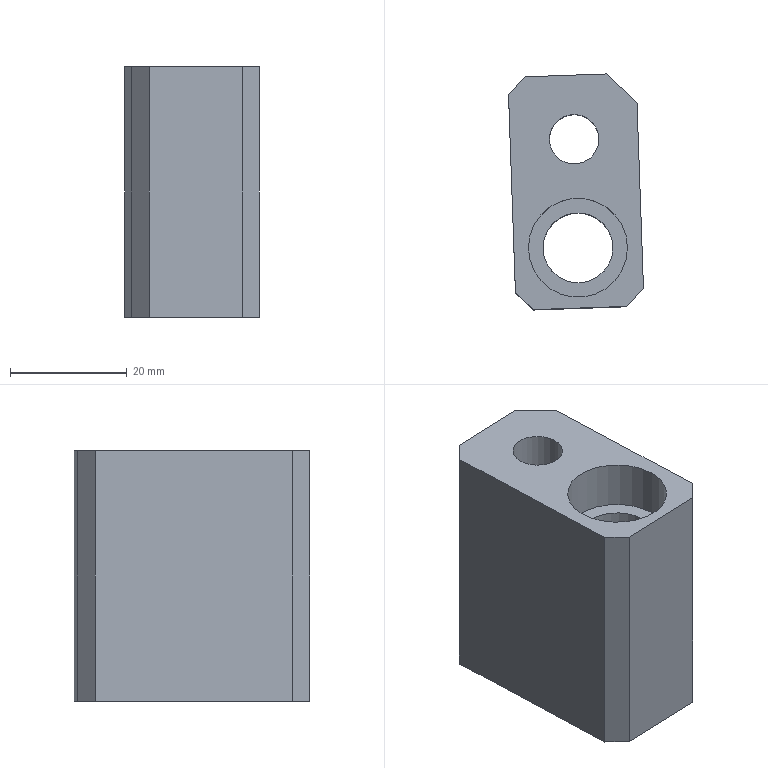Part | NX | features PH-8 2 | 1 solid | 16 faces | box 23.173 x 40.464 x 43 mm | volume 27281 mm3 | plane 12 | cylinder 4 | commonest cylinder face diameters 8.5 x1 12.001 x1 14.5 x1 17 x1
STEP:
#1=CARTESIAN_POINT('',(3121.766,-809.537,945.716));
#2=VERTEX_POINT('',#1);
#3=CARTESIAN_POINT('',(3113.266,-809.537,945.716));
#4=DIRECTION('',(0.,0.,1.));
#5=DIRECTION('',(1.,0.,0.));
#6=AXIS2_PLACEMENT_3D('',#3,#4,#5);
#7=CIRCLE('',#6,8.5);
#8=EDGE_CURVE('',#2,#2,#7,.F.);
#9=ORIENTED_EDGE('',*,*,#8,.T.);
#10=EDGE_LOOP('',(#9));
#11=FACE_BOUND('',#10,.T.);
#12=CARTESIAN_POINT('',(3116.862,-790.75,945.716));
#13=VERTEX_POINT('',#12);
#14=CARTESIAN_POINT('',(3112.615,-790.899,945.716));
#15=DIRECTION('',(0.,0.,1.));
#16=DIRECTION('',(0.9994,0.0349,0.));
#17=AXIS2_PLACEMENT_3D('',#14,#15,#16);
#18=CIRCLE('',#17,4.25);
#19=EDGE_CURVE('',#13,#13,#18,.T.);
#20=ORIENTED_EDGE('',*,*,#19,.F.);
#21=EDGE_LOOP('',(#20));
#22=FACE_BOUND('',#21,.T.);
#23=CARTESIAN_POINT('',(3123.399,-784.519,945.716));
#24=VERTEX_POINT('',#23);
#25=CARTESIAN_POINT('',(3124.515,-816.499,945.716));
#26=VERTEX_POINT('',#25);
#27=CARTESIAN_POINT('',(3123.922,-799.509,945.716));
#28=DIRECTION('',(0.0349,-0.9994,0.));
#29=VECTOR('',#28,1000.);
#30=LINE('',#27,#29);
#31=EDGE_CURVE('',#24,#26,#30,.T.);
#32=ORIENTED_EDGE('',*,*,#31,.F.);
#33=CARTESIAN_POINT('',(3118.227,-779.696,945.716));
#34=VERTEX_POINT('',#33);
#35=CARTESIAN_POINT('',(3124.433,-785.483,945.716));
#36=DIRECTION('',(0.7314,-0.682,0.));
#37=VECTOR('',#36,1000.);
#38=LINE('',#35,#37);
#39=EDGE_CURVE('',#24,#34,#38,.F.);
#40=ORIENTED_EDGE('',*,*,#39,.T.);
#41=CARTESIAN_POINT('',(3104.236,-780.185,945.716));
#42=VERTEX_POINT('',#41);
#43=CARTESIAN_POINT('',(3112.231,-779.905,945.716));
#44=DIRECTION('',(0.9994,0.0349,0.));
#45=VECTOR('',#44,1000.);
#46=LINE('',#43,#45);
#47=EDGE_CURVE('',#42,#34,#46,.T.);
#48=ORIENTED_EDGE('',*,*,#47,.F.);
#49=CARTESIAN_POINT('',(3101.342,-783.288,945.716));
#50=VERTEX_POINT('',#49);
#51=CARTESIAN_POINT('',(3099.413,-785.356,945.716));
#52=DIRECTION('',(0.682,0.7314,0.));
#53=VECTOR('',#52,1000.);
#54=LINE('',#51,#53);
#55=EDGE_CURVE('',#42,#50,#54,.F.);
#56=ORIENTED_EDGE('',*,*,#55,.T.);
#57=CARTESIAN_POINT('',(3102.529,-817.267,945.716));
#58=VERTEX_POINT('',#57);
#59=CARTESIAN_POINT('',(3101.936,-800.277,945.716));
#60=DIRECTION('',(-0.0349,0.9994,0.));
#61=VECTOR('',#60,1000.);
#62=LINE('',#59,#61);
#63=EDGE_CURVE('',#58,#50,#62,.T.);
#64=ORIENTED_EDGE('',*,*,#63,.F.);
#65=CARTESIAN_POINT('',(3105.632,-820.16,945.716));
#66=VERTEX_POINT('',#65);
#67=CARTESIAN_POINT('',(3099.426,-814.373,945.716));
#68=DIRECTION('',(-0.7314,0.682,0.));
#69=VECTOR('',#68,1000.);
#70=LINE('',#67,#69);
#71=EDGE_CURVE('',#58,#66,#70,.F.);
#72=ORIENTED_EDGE('',*,*,#71,.T.);
#73=CARTESIAN_POINT('',(3121.622,-819.602,945.716));
#74=VERTEX_POINT('',#73);
#75=CARTESIAN_POINT('',(3113.627,-819.881,945.716));
#76=DIRECTION('',(-0.9994,-0.0349,0.));
#77=VECTOR('',#76,1000.);
#78=LINE('',#75,#77);
#79=EDGE_CURVE('',#74,#66,#78,.T.);
#80=ORIENTED_EDGE('',*,*,#79,.F.);
#81=CARTESIAN_POINT('',(3127.409,-813.396,945.716));
#82=DIRECTION('',(-0.682,-0.7314,0.));
#83=VECTOR('',#82,1000.);
#84=LINE('',#81,#83);
#85=EDGE_CURVE('',#74,#26,#84,.F.);
#86=ORIENTED_EDGE('',*,*,#85,.T.);
#87=EDGE_LOOP('',(#32,#40,#48,#56,#64,#72,#80,#86));
#88=FACE_BOUND('',#87,.T.);
#89=CARTESIAN_POINT('',(3112.929,-799.893,945.716));
#90=DIRECTION('',(0.,0.,1.));
#91=DIRECTION('',(0.9994,0.0349,0.));
#92=AXIS2_PLACEMENT_3D('',#89,#90,#91);
#93=PLANE('',#92);
#94=ADVANCED_FACE('',(#11,#22,#88),#93,.T.);
#95=CARTESIAN_POINT('',(3105.632,-820.16,902.716));
#96=VERTEX_POINT('',#95);
#97=CARTESIAN_POINT('',(3121.622,-819.602,902.716));
#98=VERTEX_POINT('',#97);
#99=CARTESIAN_POINT('',(3113.627,-819.881,902.716));
#100=DIRECTION('',(0.9994,0.0349,0.));
#101=VECTOR('',#100,1000.);
#102=LINE('',#99,#101);
#103=EDGE_CURVE('',#96,#98,#102,.T.);
#104=ORIENTED_EDGE('',*,*,#103,.T.);
#105=CARTESIAN_POINT('',(3121.622,-819.602,920.716));
#106=DIRECTION('',(0.,0.,-1.));
#107=VECTOR('',#106,1000.);
#108=LINE('',#105,#107);
#109=EDGE_CURVE('',#98,#74,#108,.F.);
#110=ORIENTED_EDGE('',*,*,#109,.T.);
#111=ORIENTED_EDGE('',*,*,#79,.T.);
#112=CARTESIAN_POINT('',(3105.632,-820.16,920.716));
#113=DIRECTION('',(0.,0.,1.));
#114=VECTOR('',#113,1000.);
#115=LINE('',#112,#114);
#116=EDGE_CURVE('',#66,#96,#115,.F.);
#117=ORIENTED_EDGE('',*,*,#116,.T.);
#118=EDGE_LOOP('',(#104,#110,#111,#117));
#119=FACE_BOUND('',#118,.T.);
#120=CARTESIAN_POINT('',(3113.627,-819.881,920.716));
#121=DIRECTION('',(0.0349,-0.9994,0.));
#122=DIRECTION('',(0.,0.,-1.));
#123=AXIS2_PLACEMENT_3D('',#120,#121,#122);
#124=PLANE('',#123);
#125=ADVANCED_FACE('',(#119),#124,.T.);
#126=ORIENTED_EDGE('',*,*,#63,.T.);
#127=CARTESIAN_POINT('',(3101.342,-783.288,902.716));
#128=VERTEX_POINT('',#127);
#129=CARTESIAN_POINT('',(3101.342,-783.288,920.716));
#130=DIRECTION('',(0.,0.,-1.));
#131=VECTOR('',#130,1000.);
#132=LINE('',#129,#131);
#133=EDGE_CURVE('',#50,#128,#132,.T.);
#134=ORIENTED_EDGE('',*,*,#133,.T.);
#135=CARTESIAN_POINT('',(3102.529,-817.267,902.716));
#136=VERTEX_POINT('',#135);
#137=CARTESIAN_POINT('',(3101.936,-800.277,902.716));
#138=DIRECTION('',(0.0349,-0.9994,0.));
#139=VECTOR('',#138,1000.);
#140=LINE('',#137,#139);
#141=EDGE_CURVE('',#128,#136,#140,.T.);
#142=ORIENTED_EDGE('',*,*,#141,.T.);
#143=CARTESIAN_POINT('',(3102.529,-817.267,920.716));
#144=DIRECTION('',(0.,0.,-1.));
#145=VECTOR('',#144,1000.);
#146=LINE('',#143,#145);
#147=EDGE_CURVE('',#136,#58,#146,.F.);
#148=ORIENTED_EDGE('',*,*,#147,.T.);
#149=EDGE_LOOP('',(#126,#134,#142,#148));
#150=FACE_BOUND('',#149,.T.);
#151=CARTESIAN_POINT('',(3101.936,-800.277,920.716));
#152=DIRECTION('',(-0.9994,-0.0349,0.));
#153=DIRECTION('',(0.,0.,1.));
#154=AXIS2_PLACEMENT_3D('',#151,#152,#153);
#155=PLANE('',#154);
#156=ADVANCED_FACE('',(#150),#155,.T.);
#157=ORIENTED_EDGE('',*,*,#47,.T.);
#158=CARTESIAN_POINT('',(3118.227,-779.696,902.716));
#159=VERTEX_POINT('',#158);
#160=CARTESIAN_POINT('',(3118.227,-779.696,920.716));
#161=DIRECTION('',(0.,0.,-1.));
#162=VECTOR('',#161,1000.);
#163=LINE('',#160,#162);
#164=EDGE_CURVE('',#34,#159,#163,.T.);
#165=ORIENTED_EDGE('',*,*,#164,.T.);
#166=CARTESIAN_POINT('',(3104.236,-780.185,902.716));
#167=VERTEX_POINT('',#166);
#168=CARTESIAN_POINT('',(3112.231,-779.905,902.716));
#169=DIRECTION('',(-0.9994,-0.0349,0.));
#170=VECTOR('',#169,1000.);
#171=LINE('',#168,#170);
#172=EDGE_CURVE('',#159,#167,#171,.T.);
#173=ORIENTED_EDGE('',*,*,#172,.T.);
#174=CARTESIAN_POINT('',(3104.236,-780.185,920.716));
#175=DIRECTION('',(0.,0.,1.));
#176=VECTOR('',#175,1000.);
#177=LINE('',#174,#176);
#178=EDGE_CURVE('',#167,#42,#177,.T.);
#179=ORIENTED_EDGE('',*,*,#178,.T.);
#180=EDGE_LOOP('',(#157,#165,#173,#179));
#181=FACE_BOUND('',#180,.T.);
#182=CARTESIAN_POINT('',(3112.231,-779.905,920.716));
#183=DIRECTION('',(-0.0349,0.9994,0.));
#184=DIRECTION('',(0.,0.,1.));
#185=AXIS2_PLACEMENT_3D('',#182,#183,#184);
#186=PLANE('',#185);
#187=ADVANCED_FACE('',(#181),#186,.T.);
#188=CARTESIAN_POINT('',(3107.265,-809.537,902.716));
#189=VERTEX_POINT('',#188);
#190=CARTESIAN_POINT('',(3113.266,-809.537,902.716));
#191=DIRECTION('',(0.,0.,-1.));
#192=DIRECTION('',(-1.,0.,0.));
#193=AXIS2_PLACEMENT_3D('',#190,#191,#192);
#194=CIRCLE('',#193,6.);
#195=EDGE_CURVE('',#189,#189,#194,.T.);
#196=ORIENTED_EDGE('',*,*,#195,.F.);
#197=EDGE_LOOP('',(#196));
#198=FACE_BOUND('',#197,.T.);
#199=CARTESIAN_POINT('',(3105.365,-790.899,902.716));
#200=VERTEX_POINT('',#199);
#201=CARTESIAN_POINT('',(3112.615,-790.899,902.716));
#202=DIRECTION('',(0.,0.,-1.));
#203=DIRECTION('',(-1.,0.,0.));
#204=AXIS2_PLACEMENT_3D('',#201,#202,#203);
#205=CIRCLE('',#204,7.25);
#206=EDGE_CURVE('',#200,#200,#205,.F.);
#207=ORIENTED_EDGE('',*,*,#206,.T.);
#208=EDGE_LOOP('',(#207));
#209=FACE_BOUND('',#208,.T.);
#210=ORIENTED_EDGE('',*,*,#172,.F.);
#211=CARTESIAN_POINT('',(3123.399,-784.519,902.716));
#212=VERTEX_POINT('',#211);
#213=CARTESIAN_POINT('',(3125.467,-786.448,902.716));
#214=DIRECTION('',(-0.7314,0.682,0.));
#215=VECTOR('',#214,1000.);
#216=LINE('',#213,#215);
#217=EDGE_CURVE('',#159,#212,#216,.F.);
#218=ORIENTED_EDGE('',*,*,#217,.T.);
#219=CARTESIAN_POINT('',(3124.515,-816.499,902.716));
#220=VERTEX_POINT('',#219);
#221=CARTESIAN_POINT('',(3123.922,-799.509,902.716));
#222=DIRECTION('',(-0.0349,0.9994,0.));
#223=VECTOR('',#222,1000.);
#224=LINE('',#221,#223);
#225=EDGE_CURVE('',#220,#212,#224,.T.);
#226=ORIENTED_EDGE('',*,*,#225,.F.);
#227=CARTESIAN_POINT('',(3127.409,-813.396,902.716));
#228=DIRECTION('',(0.682,0.7314,0.));
#229=VECTOR('',#228,1000.);
#230=LINE('',#227,#229);
#231=EDGE_CURVE('',#220,#98,#230,.F.);
#232=ORIENTED_EDGE('',*,*,#231,.T.);
#233=ORIENTED_EDGE('',*,*,#103,.F.);
#234=CARTESIAN_POINT('',(3099.426,-814.373,902.716));
#235=DIRECTION('',(0.7314,-0.682,0.));
#236=VECTOR('',#235,1000.);
#237=LINE('',#234,#236);
#238=EDGE_CURVE('',#96,#136,#237,.F.);
#239=ORIENTED_EDGE('',*,*,#238,.T.);
#240=ORIENTED_EDGE('',*,*,#141,.F.);
#241=CARTESIAN_POINT('',(3098.449,-786.39,902.716));
#242=DIRECTION('',(-0.682,-0.7314,0.));
#243=VECTOR('',#242,1000.);
#244=LINE('',#241,#243);
#245=EDGE_CURVE('',#128,#167,#244,.F.);
#246=ORIENTED_EDGE('',*,*,#245,.T.);
#247=EDGE_LOOP('',(#210,#218,#226,#232,#233,#239,#240,#246));
#248=FACE_BOUND('',#247,.T.);
#249=CARTESIAN_POINT('',(3112.929,-799.893,902.716));
#250=DIRECTION('',(0.,0.,-1.));
#251=DIRECTION('',(-0.9994,-0.0349,0.));
#252=AXIS2_PLACEMENT_3D('',#249,#250,#251);
#253=PLANE('',#252);
#254=ADVANCED_FACE('',(#198,#209,#248),#253,.T.);
#255=ORIENTED_EDGE('',*,*,#225,.T.);
#256=CARTESIAN_POINT('',(3123.399,-784.519,920.716));
#257=DIRECTION('',(0.,0.,1.));
#258=VECTOR('',#257,1000.);
#259=LINE('',#256,#258);
#260=EDGE_CURVE('',#212,#24,#259,.T.);
#261=ORIENTED_EDGE('',*,*,#260,.T.);
#262=ORIENTED_EDGE('',*,*,#31,.T.);
#263=CARTESIAN_POINT('',(3124.515,-816.499,920.716));
#264=DIRECTION('',(0.,0.,1.));
#265=VECTOR('',#264,1000.);
#266=LINE('',#263,#265);
#267=EDGE_CURVE('',#26,#220,#266,.F.);
#268=ORIENTED_EDGE('',*,*,#267,.T.);
#269=EDGE_LOOP('',(#255,#261,#262,#268));
#270=FACE_BOUND('',#269,.T.);
#271=CARTESIAN_POINT('',(3123.922,-799.509,920.716));
#272=DIRECTION('',(0.9994,0.0349,0.));
#273=DIRECTION('',(0.,0.,-1.));
#274=AXIS2_PLACEMENT_3D('',#271,#272,#273);
#275=PLANE('',#274);
#276=ADVANCED_FACE('',(#270),#275,.T.);
#277=ORIENTED_EDGE('',*,*,#231,.F.);
#278=ORIENTED_EDGE('',*,*,#267,.F.);
#279=ORIENTED_EDGE('',*,*,#85,.F.);
#280=ORIENTED_EDGE('',*,*,#109,.F.);
#281=EDGE_LOOP('',(#277,#278,#279,#280));
#282=FACE_BOUND('',#281,.T.);
#283=CARTESIAN_POINT('',(3121.622,-819.602,920.716));
#284=DIRECTION('',(-0.7314,0.682,0.));
#285=DIRECTION('',(-0.682,-0.7314,0.));
#286=AXIS2_PLACEMENT_3D('',#283,#284,#285);
#287=PLANE('',#286);
#288=ADVANCED_FACE('',(#282),#287,.F.);
#289=ORIENTED_EDGE('',*,*,#238,.F.);
#290=ORIENTED_EDGE('',*,*,#116,.F.);
#291=ORIENTED_EDGE('',*,*,#71,.F.);
#292=ORIENTED_EDGE('',*,*,#147,.F.);
#293=EDGE_LOOP('',(#289,#290,#291,#292));
#294=FACE_BOUND('',#293,.T.);
#295=CARTESIAN_POINT('',(3102.529,-817.267,920.716));
#296=DIRECTION('',(0.682,0.7314,0.));
#297=DIRECTION('',(-0.7314,0.682,0.));
#298=AXIS2_PLACEMENT_3D('',#295,#296,#297);
#299=PLANE('',#298);
#300=ADVANCED_FACE('',(#294),#299,.F.);
#301=ORIENTED_EDGE('',*,*,#245,.F.);
#302=ORIENTED_EDGE('',*,*,#133,.F.);
#303=ORIENTED_EDGE('',*,*,#55,.F.);
#304=ORIENTED_EDGE('',*,*,#178,.F.);
#305=EDGE_LOOP('',(#301,#302,#303,#304));
#306=FACE_BOUND('',#305,.T.);
#307=CARTESIAN_POINT('',(3104.236,-780.185,920.716));
#308=DIRECTION('',(0.7314,-0.682,0.));
#309=DIRECTION('',(0.682,0.7314,0.));
#310=AXIS2_PLACEMENT_3D('',#307,#308,#309);
#311=PLANE('',#310);
#312=ADVANCED_FACE('',(#306),#311,.F.);
#313=CARTESIAN_POINT('',(3116.865,-790.899,913.716));
#314=VERTEX_POINT('',#313);
#315=CARTESIAN_POINT('',(3112.615,-790.899,913.716));
#316=DIRECTION('',(0.,0.,1.));
#317=DIRECTION('',(1.,0.,0.));
#318=AXIS2_PLACEMENT_3D('',#315,#316,#317);
#319=CIRCLE('',#318,4.25);
#320=EDGE_CURVE('',#314,#314,#319,.T.);
#321=ORIENTED_EDGE('',*,*,#320,.T.);
#322=EDGE_LOOP('',(#321));
#323=FACE_BOUND('',#322,.T.);
#324=CARTESIAN_POINT('',(3119.865,-790.899,913.716));
#325=VERTEX_POINT('',#324);
#326=CARTESIAN_POINT('',(3112.615,-790.899,913.716));
#327=DIRECTION('',(0.,0.,1.));
#328=DIRECTION('',(1.,0.,0.));
#329=AXIS2_PLACEMENT_3D('',#326,#327,#328);
#330=CIRCLE('',#329,7.25);
#331=EDGE_CURVE('',#325,#325,#330,.T.);
#332=ORIENTED_EDGE('',*,*,#331,.F.);
#333=EDGE_LOOP('',(#332));
#334=FACE_BOUND('',#333,.T.);
#335=CARTESIAN_POINT('',(3112.615,-790.899,913.716));
#336=DIRECTION('',(0.,0.,1.));
#337=DIRECTION('',(0.9994,0.0349,0.));
#338=AXIS2_PLACEMENT_3D('',#335,#336,#337);
#339=PLANE('',#338);
#340=ADVANCED_FACE('',(#323,#334),#339,.F.);
#341=ORIENTED_EDGE('',*,*,#206,.F.);
#342=EDGE_LOOP('',(#341));
#343=FACE_BOUND('',#342,.T.);
#344=ORIENTED_EDGE('',*,*,#331,.T.);
#345=EDGE_LOOP('',(#344));
#346=FACE_BOUND('',#345,.T.);
#347=CARTESIAN_POINT('',(3112.615,-790.899,931.716));
#348=DIRECTION('',(0.,0.,-1.));
#349=DIRECTION('',(0.9994,0.0349,0.));
#350=AXIS2_PLACEMENT_3D('',#347,#348,#349);
#351=CYLINDRICAL_SURFACE('',#350,7.25);
#352=ADVANCED_FACE('',(#343,#346),#351,.F.);
#353=ORIENTED_EDGE('',*,*,#19,.T.);
#354=EDGE_LOOP('',(#353));
#355=FACE_BOUND('',#354,.T.);
#356=ORIENTED_EDGE('',*,*,#320,.F.);
#357=EDGE_LOOP('',(#356));
#358=FACE_BOUND('',#357,.T.);
#359=CARTESIAN_POINT('',(3112.615,-790.899,946.716));
#360=DIRECTION('',(0.,0.,-1.));
#361=DIRECTION('',(0.9994,0.0349,0.));
#362=AXIS2_PLACEMENT_3D('',#359,#360,#361);
#363=CYLINDRICAL_SURFACE('',#362,4.25);
#364=ADVANCED_FACE('',(#355,#358),#363,.F.);
#365=ORIENTED_EDGE('',*,*,#195,.T.);
#366=EDGE_LOOP('',(#365));
#367=FACE_BOUND('',#366,.T.);
#368=CARTESIAN_POINT('',(3107.265,-809.537,937.416));
#369=VERTEX_POINT('',#368);
#370=CARTESIAN_POINT('',(3113.266,-809.537,937.416));
#371=DIRECTION('',(0.,0.,-1.));
#372=DIRECTION('',(-1.,0.,0.));
#373=AXIS2_PLACEMENT_3D('',#370,#371,#372);
#374=CIRCLE('',#373,6.);
#375=EDGE_CURVE('',#369,#369,#374,.T.);
#376=ORIENTED_EDGE('',*,*,#375,.F.);
#377=EDGE_LOOP('',(#376));
#378=FACE_BOUND('',#377,.T.);
#379=CARTESIAN_POINT('',(3113.266,-809.537,945.716));
#380=DIRECTION('',(0.,0.,-1.));
#381=DIRECTION('',(1.,0.,0.));
#382=AXIS2_PLACEMENT_3D('',#379,#380,#381);
#383=CYLINDRICAL_SURFACE('',#382,6.);
#384=ADVANCED_FACE('',(#367,#378),#383,.F.);
#385=ORIENTED_EDGE('',*,*,#375,.T.);
#386=EDGE_LOOP('',(#385));
#387=FACE_BOUND('',#386,.T.);
#388=CARTESIAN_POINT('',(3104.766,-809.537,937.416));
#389=VERTEX_POINT('',#388);
#390=CARTESIAN_POINT('',(3113.266,-809.537,937.416));
#391=DIRECTION('',(0.,0.,-1.));
#392=DIRECTION('',(-1.,0.,0.));
#393=AXIS2_PLACEMENT_3D('',#390,#391,#392);
#394=CIRCLE('',#393,8.5);
#395=EDGE_CURVE('',#389,#389,#394,.T.);
#396=ORIENTED_EDGE('',*,*,#395,.F.);
#397=EDGE_LOOP('',(#396));
#398=FACE_BOUND('',#397,.T.);
#399=CARTESIAN_POINT('',(3113.266,-809.537,937.416));
#400=DIRECTION('',(0.,0.,-1.));
#401=DIRECTION('',(-1.,0.,0.));
#402=AXIS2_PLACEMENT_3D('',#399,#400,#401);
#403=PLANE('',#402);
#404=ADVANCED_FACE('',(#387,#398),#403,.F.);
#405=ORIENTED_EDGE('',*,*,#395,.T.);
#406=EDGE_LOOP('',(#405));
#407=FACE_BOUND('',#406,.T.);
#408=ORIENTED_EDGE('',*,*,#8,.F.);
#409=EDGE_LOOP('',(#408));
#410=FACE_BOUND('',#409,.T.);
#411=CARTESIAN_POINT('',(3113.266,-809.537,945.716));
#412=DIRECTION('',(0.,0.,-1.));
#413=DIRECTION('',(1.,0.,0.));
#414=AXIS2_PLACEMENT_3D('',#411,#412,#413);
#415=CYLINDRICAL_SURFACE('',#414,8.5);
#416=ADVANCED_FACE('',(#407,#410),#415,.F.);
#417=ORIENTED_EDGE('',*,*,#39,.F.);
#418=ORIENTED_EDGE('',*,*,#260,.F.);
#419=ORIENTED_EDGE('',*,*,#217,.F.);
#420=ORIENTED_EDGE('',*,*,#164,.F.);
#421=EDGE_LOOP('',(#417,#418,#419,#420));
#422=FACE_BOUND('',#421,.T.);
#423=CARTESIAN_POINT('',(3118.227,-779.696,920.716));
#424=DIRECTION('',(-0.682,-0.7314,0.));
#425=DIRECTION('',(0.,0.,-1.));
#426=AXIS2_PLACEMENT_3D('',#423,#424,#425);
#427=PLANE('',#426);
#428=ADVANCED_FACE('',(#422),#427,.F.);
#429=CLOSED_SHELL('',(#94,#125,#156,#187,#254,#276,#288,#300,#312,#340,#352,#364,#384,#404,#416,#428));
#430=MANIFOLD_SOLID_BREP('',#429);
#431=(LENGTH_UNIT()NAMED_UNIT(*)SI_UNIT(.MILLI.,.METRE.));
#432=UNCERTAINTY_MEASURE_WITH_UNIT(LENGTH_MEASURE(0.00001),#431,'','');
#433=(NAMED_UNIT(*)PLANE_ANGLE_UNIT()SI_UNIT($,.RADIAN.));
#434=(NAMED_UNIT(*)SI_UNIT($,.STERADIAN.)SOLID_ANGLE_UNIT());
#435=(GEOMETRIC_REPRESENTATION_CONTEXT(3)GLOBAL_UNCERTAINTY_ASSIGNED_CONTEXT((#432))GLOBAL_UNIT_ASSIGNED_CONTEXT((#431,#433,#434))REPRESENTATION_CONTEXT('',''));
#436=ADVANCED_BREP_SHAPE_REPRESENTATION('',(#430),#435);